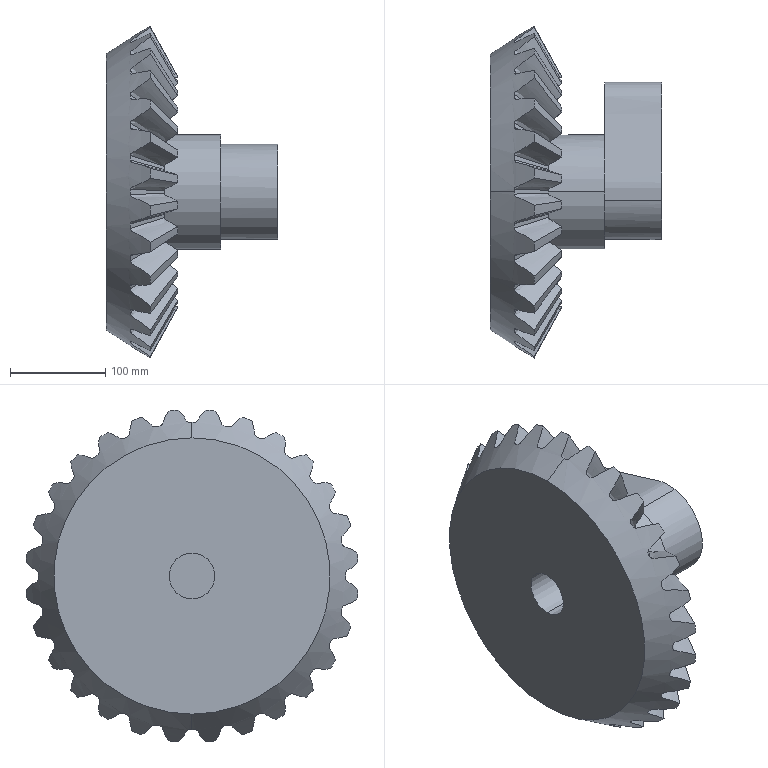Part | SolidWorks | features 3DProfileFeature 12, ICE 2, BlendCut 1, CirPattern 1, RefAxis 1, Revolution 1 | 1 solid | 128 faces | box 180.071 x 347.819 x 347.819 mm | volume 5839211 mm3 | spline 58 | plane 34 | cone 32 | cylinder 4 | commonest cylinder face diameters 47.944 x2 120 x2